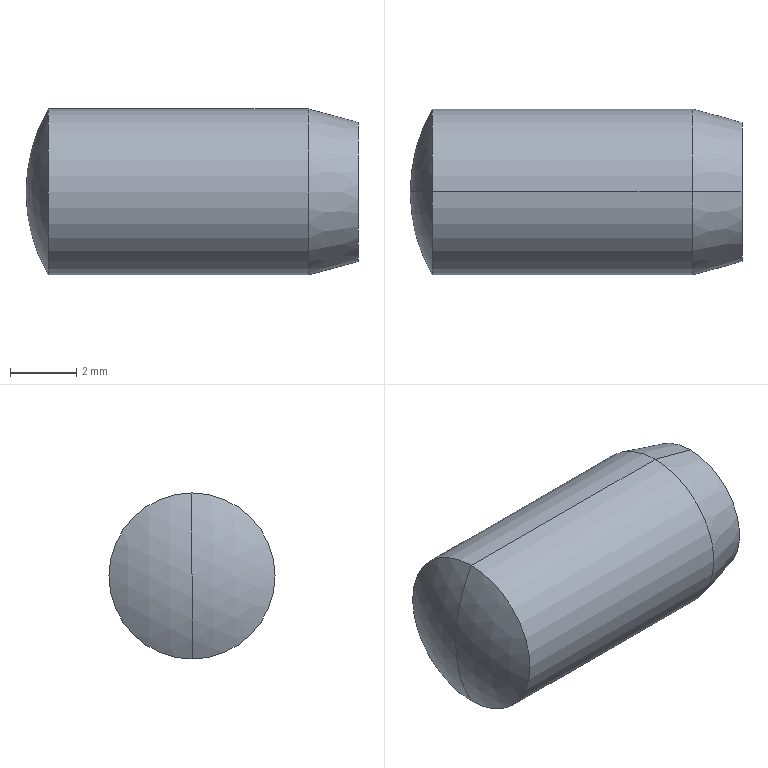Part | SolidWorks | features Revolution 1 | 1 solid | 7 faces | box 10 x 5 x 5 mm | volume 185.449 mm3 | cone 2 | cylinder 2 | sphere 2 | plane 1 | commonest cylinder face diameters 5 x2
STEP:
#1=CARTESIAN_POINT('',(0.,0.,2.098));
#2=VERTEX_POINT('',#1);
#3=CARTESIAN_POINT('',(0.,0.,-2.098));
#4=VERTEX_POINT('',#3);
#5=CARTESIAN_POINT('',(0.,0.,0.));
#6=DIRECTION('',(-1.,0.,0.));
#7=DIRECTION('',(0.,0.,1.));
#8=AXIS2_PLACEMENT_3D('',#5,#6,#7);
#9=CIRCLE('',#8,2.098);
#10=EDGE_CURVE('',#2,#4,#9,.T.);
#11=ORIENTED_EDGE('',*,*,#10,.T.);
#12=CARTESIAN_POINT('',(-1.5,0.,-2.5));
#13=VERTEX_POINT('',#12);
#14=CARTESIAN_POINT('',(-1.5,0.,-2.5));
#15=DIRECTION('',(-0.9659,0.,-0.2588));
#16=VECTOR('',#15,1000.);
#17=LINE('',#14,#16);
#18=EDGE_CURVE('',#4,#13,#17,.T.);
#19=ORIENTED_EDGE('',*,*,#18,.T.);
#20=CARTESIAN_POINT('',(-1.5,0.,2.5));
#21=VERTEX_POINT('',#20);
#22=CARTESIAN_POINT('',(-1.5,0.,0.));
#23=DIRECTION('',(-1.,0.,0.));
#24=DIRECTION('',(0.,0.,1.));
#25=AXIS2_PLACEMENT_3D('',#22,#23,#24);
#26=CIRCLE('',#25,2.5);
#27=EDGE_CURVE('',#21,#13,#26,.T.);
#28=ORIENTED_EDGE('',*,*,#27,.F.);
#29=CARTESIAN_POINT('',(-1.5,0.,2.5));
#30=DIRECTION('',(-0.9659,0.,0.2588));
#31=VECTOR('',#30,1000.);
#32=LINE('',#29,#31);
#33=EDGE_CURVE('',#2,#21,#32,.T.);
#34=ORIENTED_EDGE('',*,*,#33,.F.);
#35=EDGE_LOOP('',(#11,#19,#28,#34));
#36=FACE_OUTER_BOUND('',#35,.T.);
#37=CARTESIAN_POINT('',(-1.5,0.,0.));
#38=DIRECTION('',(-1.,0.,0.));
#39=DIRECTION('',(0.,0.,1.));
#40=AXIS2_PLACEMENT_3D('',#37,#38,#39);
#41=CONICAL_SURFACE('',#40,2.5,0.2618);
#42=ADVANCED_FACE('',(#36),#41,.T.);
#43=ORIENTED_EDGE('',*,*,#27,.T.);
#44=CARTESIAN_POINT('',(-9.33,0.,-2.5));
#45=VERTEX_POINT('',#44);
#46=CARTESIAN_POINT('',(-11.391,0.,-2.5));
#47=DIRECTION('',(-1.,0.,0.));
#48=VECTOR('',#47,1000.);
#49=LINE('',#46,#48);
#50=EDGE_CURVE('',#13,#45,#49,.T.);
#51=ORIENTED_EDGE('',*,*,#50,.T.);
#52=CARTESIAN_POINT('',(-9.33,0.,2.5));
#53=VERTEX_POINT('',#52);
#54=CARTESIAN_POINT('',(-9.33,0.,0.));
#55=DIRECTION('',(-1.,0.,0.));
#56=DIRECTION('',(0.,0.,1.));
#57=AXIS2_PLACEMENT_3D('',#54,#55,#56);
#58=CIRCLE('',#57,2.5);
#59=EDGE_CURVE('',#53,#45,#58,.T.);
#60=ORIENTED_EDGE('',*,*,#59,.F.);
#61=CARTESIAN_POINT('',(-11.391,0.,2.5));
#62=DIRECTION('',(-1.,0.,0.));
#63=VECTOR('',#62,1000.);
#64=LINE('',#61,#63);
#65=EDGE_CURVE('',#21,#53,#64,.T.);
#66=ORIENTED_EDGE('',*,*,#65,.F.);
#67=EDGE_LOOP('',(#43,#51,#60,#66));
#68=FACE_OUTER_BOUND('',#67,.T.);
#69=CARTESIAN_POINT('',(-11.391,0.,0.));
#70=DIRECTION('',(-1.,0.,0.));
#71=DIRECTION('',(0.,0.,1.));
#72=AXIS2_PLACEMENT_3D('',#69,#70,#71);
#73=CYLINDRICAL_SURFACE('',#72,2.5);
#74=ADVANCED_FACE('',(#68),#73,.T.);
#75=CARTESIAN_POINT('',(-9.33,0.,0.));
#76=DIRECTION('',(-1.,0.,0.));
#77=DIRECTION('',(0.,0.,1.));
#78=AXIS2_PLACEMENT_3D('',#75,#76,#77);
#79=CIRCLE('',#78,2.5);
#80=EDGE_CURVE('',#45,#53,#79,.T.);
#81=ORIENTED_EDGE('',*,*,#80,.T.);
#82=CARTESIAN_POINT('',(-10.,0.,0.));
#83=VERTEX_POINT('',#82);
#84=CARTESIAN_POINT('',(-5.,0.,0.));
#85=DIRECTION('',(0.,-1.,0.));
#86=DIRECTION('',(0.,0.,-1.));
#87=AXIS2_PLACEMENT_3D('',#84,#85,#86);
#88=CIRCLE('',#87,5.);
#89=EDGE_CURVE('',#53,#83,#88,.T.);
#90=ORIENTED_EDGE('',*,*,#89,.T.);
#91=CARTESIAN_POINT('',(-5.,0.,0.));
#92=DIRECTION('',(0.,1.,0.));
#93=DIRECTION('',(0.,0.,1.));
#94=AXIS2_PLACEMENT_3D('',#91,#92,#93);
#95=CIRCLE('',#94,5.);
#96=EDGE_CURVE('',#45,#83,#95,.T.);
#97=ORIENTED_EDGE('',*,*,#96,.F.);
#98=EDGE_LOOP('',(#81,#90,#97));
#99=FACE_OUTER_BOUND('',#98,.T.);
#100=CARTESIAN_POINT('',(-5.,0.,0.));
#101=DIRECTION('',(0.,-1.,0.));
#102=DIRECTION('',(0.,0.,-1.));
#103=AXIS2_PLACEMENT_3D('',#100,#101,#102);
#104=SPHERICAL_SURFACE('',#103,5.);
#105=ADVANCED_FACE('',(#99),#104,.T.);
#106=ORIENTED_EDGE('',*,*,#10,.F.);
#107=CARTESIAN_POINT('',(0.,0.,0.));
#108=DIRECTION('',(-1.,0.,0.));
#109=DIRECTION('',(0.,0.,1.));
#110=AXIS2_PLACEMENT_3D('',#107,#108,#109);
#111=CIRCLE('',#110,2.098);
#112=EDGE_CURVE('',#4,#2,#111,.T.);
#113=ORIENTED_EDGE('',*,*,#112,.F.);
#114=EDGE_LOOP('',(#106,#113));
#115=FACE_OUTER_BOUND('',#114,.T.);
#116=CARTESIAN_POINT('',(0.,0.,0.));
#117=DIRECTION('',(1.,0.,0.));
#118=DIRECTION('',(0.,0.,-1.));
#119=AXIS2_PLACEMENT_3D('',#116,#117,#118);
#120=PLANE('',#119);
#121=ADVANCED_FACE('',(#115),#120,.T.);
#122=ORIENTED_EDGE('',*,*,#89,.F.);
#123=ORIENTED_EDGE('',*,*,#59,.T.);
#124=ORIENTED_EDGE('',*,*,#96,.T.);
#125=EDGE_LOOP('',(#122,#123,#124));
#126=FACE_OUTER_BOUND('',#125,.T.);
#127=CARTESIAN_POINT('',(-5.,0.,0.));
#128=DIRECTION('',(0.,-1.,0.));
#129=DIRECTION('',(0.,0.,-1.));
#130=AXIS2_PLACEMENT_3D('',#127,#128,#129);
#131=SPHERICAL_SURFACE('',#130,5.);
#132=ADVANCED_FACE('',(#126),#131,.T.);
#133=ORIENTED_EDGE('',*,*,#50,.F.);
#134=CARTESIAN_POINT('',(-1.5,0.,0.));
#135=DIRECTION('',(-1.,0.,0.));
#136=DIRECTION('',(0.,0.,1.));
#137=AXIS2_PLACEMENT_3D('',#134,#135,#136);
#138=CIRCLE('',#137,2.5);
#139=EDGE_CURVE('',#13,#21,#138,.T.);
#140=ORIENTED_EDGE('',*,*,#139,.T.);
#141=ORIENTED_EDGE('',*,*,#65,.T.);
#142=ORIENTED_EDGE('',*,*,#80,.F.);
#143=EDGE_LOOP('',(#133,#140,#141,#142));
#144=FACE_OUTER_BOUND('',#143,.T.);
#145=CARTESIAN_POINT('',(-11.391,0.,0.));
#146=DIRECTION('',(-1.,0.,0.));
#147=DIRECTION('',(0.,0.,1.));
#148=AXIS2_PLACEMENT_3D('',#145,#146,#147);
#149=CYLINDRICAL_SURFACE('',#148,2.5);
#150=ADVANCED_FACE('',(#144),#149,.T.);
#151=ORIENTED_EDGE('',*,*,#18,.F.);
#152=ORIENTED_EDGE('',*,*,#112,.T.);
#153=ORIENTED_EDGE('',*,*,#33,.T.);
#154=ORIENTED_EDGE('',*,*,#139,.F.);
#155=EDGE_LOOP('',(#151,#152,#153,#154));
#156=FACE_OUTER_BOUND('',#155,.T.);
#157=CARTESIAN_POINT('',(-1.5,0.,0.));
#158=DIRECTION('',(-1.,0.,0.));
#159=DIRECTION('',(0.,0.,1.));
#160=AXIS2_PLACEMENT_3D('',#157,#158,#159);
#161=CONICAL_SURFACE('',#160,2.5,0.2618);
#162=ADVANCED_FACE('',(#156),#161,.T.);
#163=CLOSED_SHELL('',(#42,#74,#105,#121,#132,#150,#162));
#164=MANIFOLD_SOLID_BREP('',#163);
#165=CARTESIAN_POINT('',(0.,0.,0.));
#166=DIRECTION('',(0.,0.,1.));
#167=DIRECTION('',(1.,0.,0.));
#168=AXIS2_PLACEMENT_3D('',#165,#166,#167);
#169=(LENGTH_UNIT()NAMED_UNIT(*)SI_UNIT(.MILLI.,.METRE.));
#170=UNCERTAINTY_MEASURE_WITH_UNIT(LENGTH_MEASURE(0.00001),#169,'','');
#171=(NAMED_UNIT(*)PLANE_ANGLE_UNIT()SI_UNIT($,.RADIAN.));
#172=(NAMED_UNIT(*)SI_UNIT($,.STERADIAN.)SOLID_ANGLE_UNIT());
#173=(GEOMETRIC_REPRESENTATION_CONTEXT(3)GLOBAL_UNCERTAINTY_ASSIGNED_CONTEXT((#170))GLOBAL_UNIT_ASSIGNED_CONTEXT((#169,#171,#172))REPRESENTATION_CONTEXT('',''));
#174=ADVANCED_BREP_SHAPE_REPRESENTATION('',(#164,#168),#173);